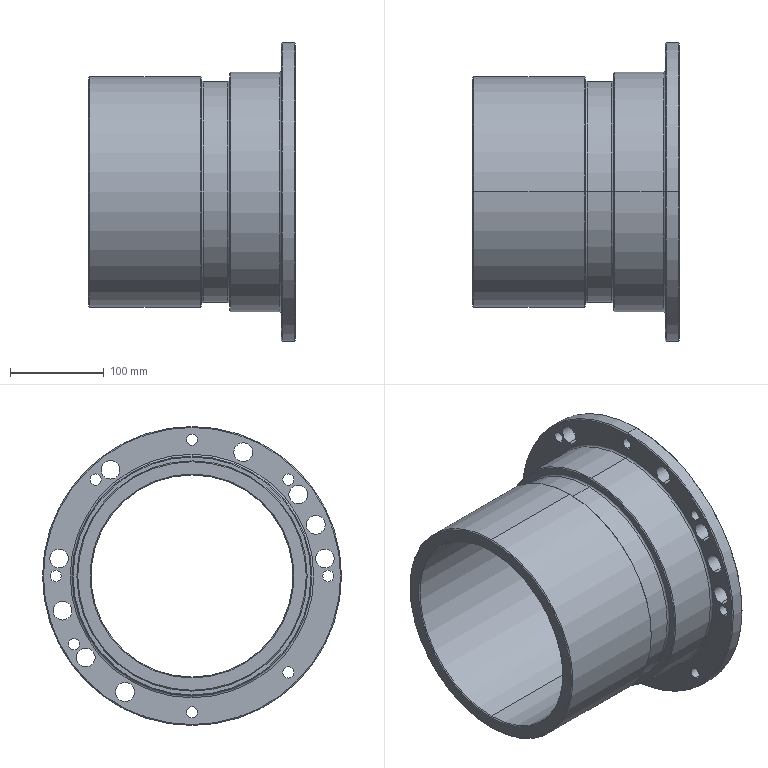Part | SolidWorks | features Chamfer 2, Fillet 2, ICE 2, Revolution 1 | 1 solid | 83 faces | box 220 x 318 x 318 mm | volume 2874143 mm3 | cylinder 48 | cone 14 | torus 14 | plane 7 | commonest cylinder face diameters 20 x18 12 x16 215 x2 224.6 x2 235 x2 244 x2